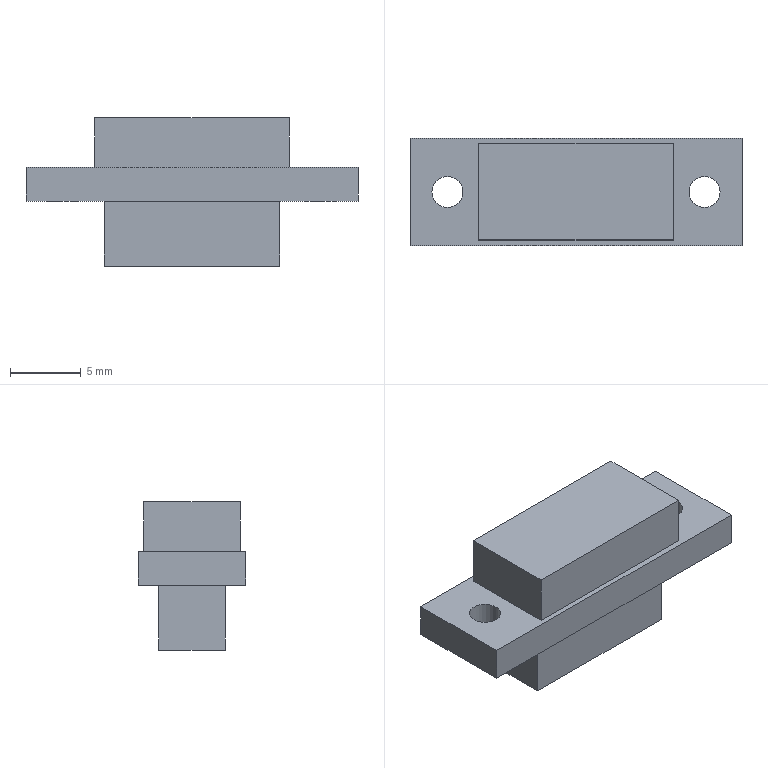Part | STEP file | J30J-15ZKP | 1 solid | 23 faces | box 23.5 x 7.6 x 10.5 mm | volume 877.754 mm3 | plane 21 | cylinder 2 | commonest cylinder face diameters 2.2 x2